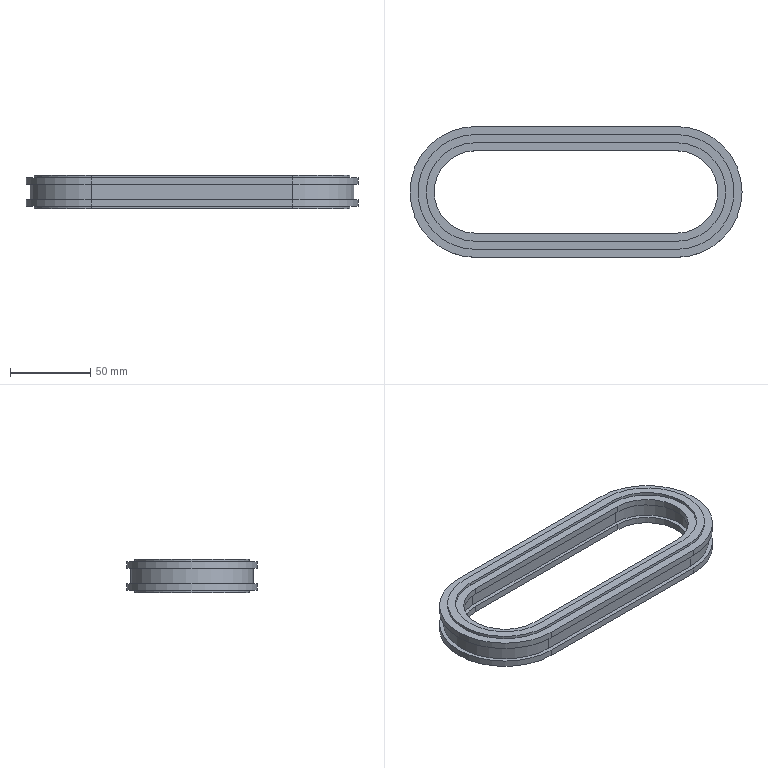Part | STEP file | Roller chain_1 | 1 solid | 50 faces | box 206.346 x 81.346 x 21.082 mm | volume 108276 mm3 | plane 30 | cylinder 20 | commonest cylinder face diameters 51.324 x4 61.255 x4 71.415 x4 81.346 x4 56.175 x2 76.495 x2